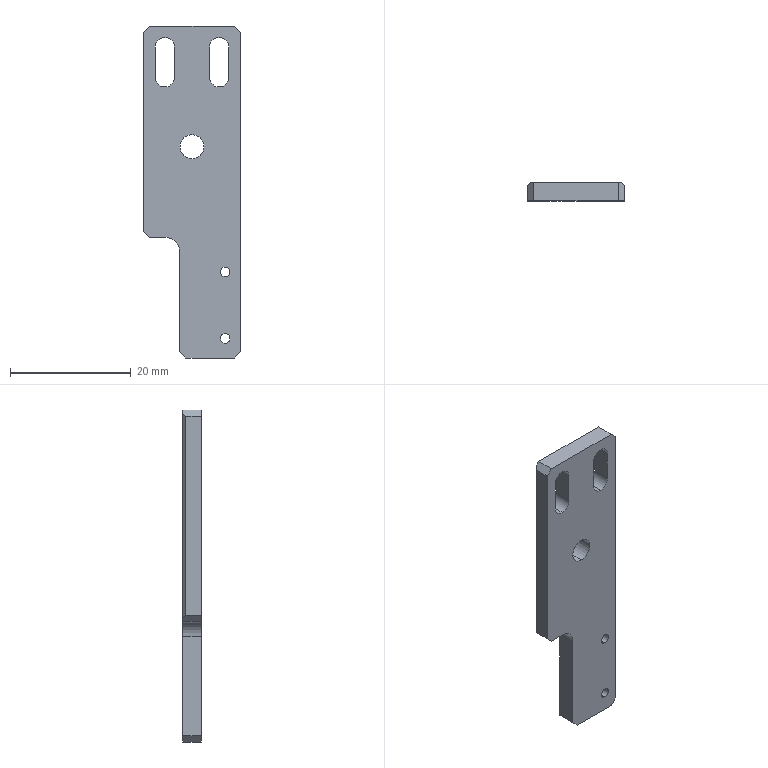Part | SolidWorks | features Chamfer 2, HoleWzd 2, Cut 1, Extrusion 1, Fillet 1, ICE 1 | 1 solid | 32 faces | box 16 x 3 x 55 mm | volume 2072 mm3 | plane 19 | cylinder 13 | commonest cylinder face diameters 3.2 x6 1.6 x4 4 x2 5 x1
STEP:
#1=CARTESIAN_POINT('',(8.,3.,33.));
#2=VERTEX_POINT('',#1);
#3=CARTESIAN_POINT('',(8.,3.,37.));
#4=VERTEX_POINT('',#3);
#5=CARTESIAN_POINT('',(8.,3.,35.));
#6=DIRECTION('',(0.,1.,0.));
#7=DIRECTION('',(0.,0.,1.));
#8=AXIS2_PLACEMENT_3D('',#5,#6,#7);
#9=CIRCLE('',#8,2.);
#10=EDGE_CURVE('',#2,#4,#9,.T.);
#11=ORIENTED_EDGE('',*,*,#10,.T.);
#12=CARTESIAN_POINT('',(8.,0.,37.));
#13=VERTEX_POINT('',#12);
#14=CARTESIAN_POINT('',(8.,0.,37.));
#15=DIRECTION('',(0.,-1.,0.));
#16=VECTOR('',#15,1000.);
#17=LINE('',#14,#16);
#18=EDGE_CURVE('',#4,#13,#17,.T.);
#19=ORIENTED_EDGE('',*,*,#18,.T.);
#20=CARTESIAN_POINT('',(8.,0.,33.));
#21=VERTEX_POINT('',#20);
#22=CARTESIAN_POINT('',(8.,0.,35.));
#23=DIRECTION('',(0.,-1.,0.));
#24=DIRECTION('',(0.,0.,-1.));
#25=AXIS2_PLACEMENT_3D('',#22,#23,#24);
#26=CIRCLE('',#25,2.);
#27=EDGE_CURVE('',#13,#21,#26,.T.);
#28=ORIENTED_EDGE('',*,*,#27,.T.);
#29=CARTESIAN_POINT('',(8.,0.,33.));
#30=DIRECTION('',(0.,-1.,0.));
#31=VECTOR('',#30,1000.);
#32=LINE('',#29,#31);
#33=EDGE_CURVE('',#2,#21,#32,.T.);
#34=ORIENTED_EDGE('',*,*,#33,.F.);
#35=EDGE_LOOP('',(#11,#19,#28,#34));
#36=FACE_OUTER_BOUND('',#35,.T.);
#37=CARTESIAN_POINT('',(8.,0.,35.));
#38=DIRECTION('',(0.,-1.,0.));
#39=DIRECTION('',(0.,0.,-1.));
#40=AXIS2_PLACEMENT_3D('',#37,#38,#39);
#41=CYLINDRICAL_SURFACE('',#40,2.);
#42=ADVANCED_FACE('',(#36),#41,.F.);
#43=CARTESIAN_POINT('',(13.5,0.,2.45));
#44=VERTEX_POINT('',#43);
#45=CARTESIAN_POINT('',(13.5,0.,4.05));
#46=VERTEX_POINT('',#45);
#47=CARTESIAN_POINT('',(13.5,0.,3.25));
#48=DIRECTION('',(0.,1.,0.));
#49=DIRECTION('',(0.,0.,1.));
#50=AXIS2_PLACEMENT_3D('',#47,#48,#49);
#51=CIRCLE('',#50,0.8);
#52=EDGE_CURVE('',#44,#46,#51,.T.);
#53=ORIENTED_EDGE('',*,*,#52,.F.);
#54=CARTESIAN_POINT('',(13.5,3.,2.45));
#55=VERTEX_POINT('',#54);
#56=CARTESIAN_POINT('',(13.5,3.,2.45));
#57=DIRECTION('',(0.,1.,0.));
#58=VECTOR('',#57,1000.);
#59=LINE('',#56,#58);
#60=EDGE_CURVE('',#44,#55,#59,.T.);
#61=ORIENTED_EDGE('',*,*,#60,.T.);
#62=CARTESIAN_POINT('',(13.5,3.,4.05));
#63=VERTEX_POINT('',#62);
#64=CARTESIAN_POINT('',(13.5,3.,3.25));
#65=DIRECTION('',(0.,1.,0.));
#66=DIRECTION('',(0.,0.,1.));
#67=AXIS2_PLACEMENT_3D('',#64,#65,#66);
#68=CIRCLE('',#67,0.8);
#69=EDGE_CURVE('',#55,#63,#68,.T.);
#70=ORIENTED_EDGE('',*,*,#69,.T.);
#71=CARTESIAN_POINT('',(13.5,3.,4.05));
#72=DIRECTION('',(0.,1.,0.));
#73=VECTOR('',#72,1000.);
#74=LINE('',#71,#73);
#75=EDGE_CURVE('',#46,#63,#74,.T.);
#76=ORIENTED_EDGE('',*,*,#75,.F.);
#77=EDGE_LOOP('',(#53,#61,#70,#76));
#78=FACE_OUTER_BOUND('',#77,.T.);
#79=CARTESIAN_POINT('',(13.5,3.,3.25));
#80=DIRECTION('',(0.,1.,0.));
#81=DIRECTION('',(0.,0.,1.));
#82=AXIS2_PLACEMENT_3D('',#79,#80,#81);
#83=CYLINDRICAL_SURFACE('',#82,0.8);
#84=ADVANCED_FACE('',(#78),#83,.F.);
#85=CARTESIAN_POINT('',(13.5,0.,13.45));
#86=VERTEX_POINT('',#85);
#87=CARTESIAN_POINT('',(13.5,0.,15.05));
#88=VERTEX_POINT('',#87);
#89=CARTESIAN_POINT('',(13.5,0.,14.25));
#90=DIRECTION('',(0.,1.,0.));
#91=DIRECTION('',(0.,0.,1.));
#92=AXIS2_PLACEMENT_3D('',#89,#90,#91);
#93=CIRCLE('',#92,0.8);
#94=EDGE_CURVE('',#86,#88,#93,.T.);
#95=ORIENTED_EDGE('',*,*,#94,.F.);
#96=CARTESIAN_POINT('',(13.5,3.,13.45));
#97=VERTEX_POINT('',#96);
#98=CARTESIAN_POINT('',(13.5,3.,13.45));
#99=DIRECTION('',(0.,1.,0.));
#100=VECTOR('',#99,1000.);
#101=LINE('',#98,#100);
#102=EDGE_CURVE('',#86,#97,#101,.T.);
#103=ORIENTED_EDGE('',*,*,#102,.T.);
#104=CARTESIAN_POINT('',(13.5,3.,15.05));
#105=VERTEX_POINT('',#104);
#106=CARTESIAN_POINT('',(13.5,3.,14.25));
#107=DIRECTION('',(0.,1.,0.));
#108=DIRECTION('',(0.,0.,1.));
#109=AXIS2_PLACEMENT_3D('',#106,#107,#108);
#110=CIRCLE('',#109,0.8);
#111=EDGE_CURVE('',#97,#105,#110,.T.);
#112=ORIENTED_EDGE('',*,*,#111,.T.);
#113=CARTESIAN_POINT('',(13.5,3.,15.05));
#114=DIRECTION('',(0.,1.,0.));
#115=VECTOR('',#114,1000.);
#116=LINE('',#113,#115);
#117=EDGE_CURVE('',#88,#105,#116,.T.);
#118=ORIENTED_EDGE('',*,*,#117,.F.);
#119=EDGE_LOOP('',(#95,#103,#112,#118));
#120=FACE_OUTER_BOUND('',#119,.T.);
#121=CARTESIAN_POINT('',(13.5,3.,14.25));
#122=DIRECTION('',(0.,1.,0.));
#123=DIRECTION('',(0.,0.,1.));
#124=AXIS2_PLACEMENT_3D('',#121,#122,#123);
#125=CYLINDRICAL_SURFACE('',#124,0.8);
#126=ADVANCED_FACE('',(#120),#125,.F.);
#127=CARTESIAN_POINT('',(14.1,3.,46.5));
#128=VERTEX_POINT('',#127);
#129=CARTESIAN_POINT('',(12.5,3.,44.9));
#130=VERTEX_POINT('',#129);
#131=CARTESIAN_POINT('',(12.5,3.,46.5));
#132=DIRECTION('',(0.,1.,0.));
#133=DIRECTION('',(0.,0.,1.));
#134=AXIS2_PLACEMENT_3D('',#131,#132,#133);
#135=CIRCLE('',#134,1.6);
#136=EDGE_CURVE('',#128,#130,#135,.T.);
#137=ORIENTED_EDGE('',*,*,#136,.T.);
#138=CARTESIAN_POINT('',(12.5,0.,44.9));
#139=VERTEX_POINT('',#138);
#140=CARTESIAN_POINT('',(12.5,10.,44.9));
#141=DIRECTION('',(0.,-1.,0.));
#142=VECTOR('',#141,1000.);
#143=LINE('',#140,#142);
#144=EDGE_CURVE('',#130,#139,#143,.T.);
#145=ORIENTED_EDGE('',*,*,#144,.T.);
#146=CARTESIAN_POINT('',(14.1,0.,46.5));
#147=VERTEX_POINT('',#146);
#148=CARTESIAN_POINT('',(12.5,0.,46.5));
#149=DIRECTION('',(0.,-1.,0.));
#150=DIRECTION('',(0.,0.,1.));
#151=AXIS2_PLACEMENT_3D('',#148,#149,#150);
#152=CIRCLE('',#151,1.6);
#153=EDGE_CURVE('',#139,#147,#152,.T.);
#154=ORIENTED_EDGE('',*,*,#153,.T.);
#155=CARTESIAN_POINT('',(14.1,10.,46.5));
#156=DIRECTION('',(0.,-1.,0.));
#157=VECTOR('',#156,1000.);
#158=LINE('',#155,#157);
#159=EDGE_CURVE('',#128,#147,#158,.T.);
#160=ORIENTED_EDGE('',*,*,#159,.F.);
#161=EDGE_LOOP('',(#137,#145,#154,#160));
#162=FACE_OUTER_BOUND('',#161,.T.);
#163=CARTESIAN_POINT('',(12.5,10.,46.5));
#164=DIRECTION('',(0.,-1.,0.));
#165=DIRECTION('',(0.,0.,-1.));
#166=AXIS2_PLACEMENT_3D('',#163,#164,#165);
#167=CYLINDRICAL_SURFACE('',#166,1.6);
#168=ADVANCED_FACE('',(#162),#167,.F.);
#169=CARTESIAN_POINT('',(5.1,3.,46.5));
#170=VERTEX_POINT('',#169);
#171=CARTESIAN_POINT('',(3.5,3.,44.9));
#172=VERTEX_POINT('',#171);
#173=CARTESIAN_POINT('',(3.5,3.,46.5));
#174=DIRECTION('',(0.,1.,0.));
#175=DIRECTION('',(0.,0.,1.));
#176=AXIS2_PLACEMENT_3D('',#173,#174,#175);
#177=CIRCLE('',#176,1.6);
#178=EDGE_CURVE('',#170,#172,#177,.T.);
#179=ORIENTED_EDGE('',*,*,#178,.T.);
#180=CARTESIAN_POINT('',(3.5,0.,44.9));
#181=VERTEX_POINT('',#180);
#182=CARTESIAN_POINT('',(3.5,10.,44.9));
#183=DIRECTION('',(0.,-1.,0.));
#184=VECTOR('',#183,1000.);
#185=LINE('',#182,#184);
#186=EDGE_CURVE('',#172,#181,#185,.T.);
#187=ORIENTED_EDGE('',*,*,#186,.T.);
#188=CARTESIAN_POINT('',(5.1,0.,46.5));
#189=VERTEX_POINT('',#188);
#190=CARTESIAN_POINT('',(3.5,0.,46.5));
#191=DIRECTION('',(0.,-1.,0.));
#192=DIRECTION('',(0.,0.,-1.));
#193=AXIS2_PLACEMENT_3D('',#190,#191,#192);
#194=CIRCLE('',#193,1.6);
#195=EDGE_CURVE('',#181,#189,#194,.T.);
#196=ORIENTED_EDGE('',*,*,#195,.T.);
#197=CARTESIAN_POINT('',(5.1,10.,46.5));
#198=DIRECTION('',(0.,-1.,0.));
#199=VECTOR('',#198,1000.);
#200=LINE('',#197,#199);
#201=EDGE_CURVE('',#170,#189,#200,.T.);
#202=ORIENTED_EDGE('',*,*,#201,.F.);
#203=EDGE_LOOP('',(#179,#187,#196,#202));
#204=FACE_OUTER_BOUND('',#203,.T.);
#205=CARTESIAN_POINT('',(3.5,10.,46.5));
#206=DIRECTION('',(0.,-1.,0.));
#207=DIRECTION('',(0.,0.,-1.));
#208=AXIS2_PLACEMENT_3D('',#205,#206,#207);
#209=CYLINDRICAL_SURFACE('',#208,1.6);
#210=ADVANCED_FACE('',(#204),#209,.F.);
#211=CARTESIAN_POINT('',(0.,0.,54.));
#212=VERTEX_POINT('',#211);
#213=CARTESIAN_POINT('',(0.,2.5,54.));
#214=VERTEX_POINT('',#213);
#215=CARTESIAN_POINT('',(0.,3.,54.));
#216=DIRECTION('',(0.,1.,0.));
#217=VECTOR('',#216,1000.);
#218=LINE('',#215,#217);
#219=EDGE_CURVE('',#212,#214,#218,.T.);
#220=ORIENTED_EDGE('',*,*,#219,.T.);
#221=CARTESIAN_POINT('',(0.,2.5,21.));
#222=VERTEX_POINT('',#221);
#223=CARTESIAN_POINT('',(0.,2.5,21.));
#224=DIRECTION('',(0.,0.,-1.));
#225=VECTOR('',#224,1000.);
#226=LINE('',#223,#225);
#227=EDGE_CURVE('',#214,#222,#226,.T.);
#228=ORIENTED_EDGE('',*,*,#227,.T.);
#229=CARTESIAN_POINT('',(0.,0.,21.));
#230=VERTEX_POINT('',#229);
#231=CARTESIAN_POINT('',(0.,3.,21.));
#232=DIRECTION('',(0.,-1.,0.));
#233=VECTOR('',#232,1000.);
#234=LINE('',#231,#233);
#235=EDGE_CURVE('',#222,#230,#234,.T.);
#236=ORIENTED_EDGE('',*,*,#235,.T.);
#237=CARTESIAN_POINT('',(0.,0.,0.));
#238=DIRECTION('',(0.,0.,1.));
#239=VECTOR('',#238,1000.);
#240=LINE('',#237,#239);
#241=EDGE_CURVE('',#230,#212,#240,.T.);
#242=ORIENTED_EDGE('',*,*,#241,.T.);
#243=EDGE_LOOP('',(#220,#228,#236,#242));
#244=FACE_OUTER_BOUND('',#243,.T.);
#245=CARTESIAN_POINT('',(0.,3.,0.));
#246=DIRECTION('',(1.,0.,0.));
#247=DIRECTION('',(0.,0.,-1.));
#248=AXIS2_PLACEMENT_3D('',#245,#246,#247);
#249=PLANE('',#248);
#250=ADVANCED_FACE('',(#244),#249,.F.);
#251=CARTESIAN_POINT('',(1.,0.,55.));
#252=VERTEX_POINT('',#251);
#253=CARTESIAN_POINT('',(15.,0.,55.));
#254=VERTEX_POINT('',#253);
#255=CARTESIAN_POINT('',(0.,0.,55.));
#256=DIRECTION('',(1.,0.,0.));
#257=VECTOR('',#256,1000.);
#258=LINE('',#255,#257);
#259=EDGE_CURVE('',#252,#254,#258,.T.);
#260=ORIENTED_EDGE('',*,*,#259,.T.);
#261=CARTESIAN_POINT('',(15.,3.,55.));
#262=VERTEX_POINT('',#261);
#263=CARTESIAN_POINT('',(15.,3.,55.));
#264=DIRECTION('',(0.,1.,0.));
#265=VECTOR('',#264,1000.);
#266=LINE('',#263,#265);
#267=EDGE_CURVE('',#254,#262,#266,.T.);
#268=ORIENTED_EDGE('',*,*,#267,.T.);
#269=CARTESIAN_POINT('',(1.,3.,55.));
#270=VERTEX_POINT('',#269);
#271=CARTESIAN_POINT('',(0.,3.,55.));
#272=DIRECTION('',(1.,0.,0.));
#273=VECTOR('',#272,1000.);
#274=LINE('',#271,#273);
#275=EDGE_CURVE('',#270,#262,#274,.T.);
#276=ORIENTED_EDGE('',*,*,#275,.F.);
#277=CARTESIAN_POINT('',(1.,3.,55.));
#278=DIRECTION('',(0.,-1.,0.));
#279=VECTOR('',#278,1000.);
#280=LINE('',#277,#279);
#281=EDGE_CURVE('',#270,#252,#280,.T.);
#282=ORIENTED_EDGE('',*,*,#281,.T.);
#283=EDGE_LOOP('',(#260,#268,#276,#282));
#284=FACE_OUTER_BOUND('',#283,.T.);
#285=CARTESIAN_POINT('',(0.,3.,55.));
#286=DIRECTION('',(0.,0.,-1.));
#287=DIRECTION('',(-1.,0.,0.));
#288=AXIS2_PLACEMENT_3D('',#285,#286,#287);
#289=PLANE('',#288);
#290=ADVANCED_FACE('',(#284),#289,.F.);
#291=CARTESIAN_POINT('',(16.,0.,1.));
#292=VERTEX_POINT('',#291);
#293=CARTESIAN_POINT('',(16.,2.5,1.));
#294=VERTEX_POINT('',#293);
#295=CARTESIAN_POINT('',(16.,3.,1.));
#296=DIRECTION('',(0.,1.,0.));
#297=VECTOR('',#296,1000.);
#298=LINE('',#295,#297);
#299=EDGE_CURVE('',#292,#294,#298,.T.);
#300=ORIENTED_EDGE('',*,*,#299,.T.);
#301=CARTESIAN_POINT('',(16.,2.5,54.));
#302=VERTEX_POINT('',#301);
#303=CARTESIAN_POINT('',(16.,2.5,54.));
#304=DIRECTION('',(0.,0.,1.));
#305=VECTOR('',#304,1000.);
#306=LINE('',#303,#305);
#307=EDGE_CURVE('',#294,#302,#306,.T.);
#308=ORIENTED_EDGE('',*,*,#307,.T.);
#309=CARTESIAN_POINT('',(16.,0.,54.));
#310=VERTEX_POINT('',#309);
#311=CARTESIAN_POINT('',(16.,3.,54.));
#312=DIRECTION('',(0.,-1.,0.));
#313=VECTOR('',#312,1000.);
#314=LINE('',#311,#313);
#315=EDGE_CURVE('',#302,#310,#314,.T.);
#316=ORIENTED_EDGE('',*,*,#315,.T.);
#317=CARTESIAN_POINT('',(16.,0.,0.));
#318=DIRECTION('',(0.,0.,-1.));
#319=VECTOR('',#318,1000.);
#320=LINE('',#317,#319);
#321=EDGE_CURVE('',#310,#292,#320,.T.);
#322=ORIENTED_EDGE('',*,*,#321,.T.);
#323=EDGE_LOOP('',(#300,#308,#316,#322));
#324=FACE_OUTER_BOUND('',#323,.T.);
#325=CARTESIAN_POINT('',(16.,3.,0.));
#326=DIRECTION('',(-1.,0.,0.));
#327=DIRECTION('',(0.,0.,1.));
#328=AXIS2_PLACEMENT_3D('',#325,#326,#327);
#329=PLANE('',#328);
#330=ADVANCED_FACE('',(#324),#329,.F.);
#331=CARTESIAN_POINT('',(15.,0.,0.));
#332=VERTEX_POINT('',#331);
#333=CARTESIAN_POINT('',(7.,0.,0.));
#334=VERTEX_POINT('',#333);
#335=CARTESIAN_POINT('',(0.,0.,0.));
#336=DIRECTION('',(-1.,0.,0.));
#337=VECTOR('',#336,1000.);
#338=LINE('',#335,#337);
#339=EDGE_CURVE('',#332,#334,#338,.T.);
#340=ORIENTED_EDGE('',*,*,#339,.T.);
#341=CARTESIAN_POINT('',(7.,3.,0.));
#342=VERTEX_POINT('',#341);
#343=CARTESIAN_POINT('',(7.,3.,0.));
#344=DIRECTION('',(0.,1.,0.));
#345=VECTOR('',#344,1000.);
#346=LINE('',#343,#345);
#347=EDGE_CURVE('',#334,#342,#346,.T.);
#348=ORIENTED_EDGE('',*,*,#347,.T.);
#349=CARTESIAN_POINT('',(15.,3.,0.));
#350=VERTEX_POINT('',#349);
#351=CARTESIAN_POINT('',(0.,3.,0.));
#352=DIRECTION('',(-1.,0.,0.));
#353=VECTOR('',#352,1000.);
#354=LINE('',#351,#353);
#355=EDGE_CURVE('',#350,#342,#354,.T.);
#356=ORIENTED_EDGE('',*,*,#355,.F.);
#357=CARTESIAN_POINT('',(15.,3.,0.));
#358=DIRECTION('',(0.,-1.,0.));
#359=VECTOR('',#358,1000.);
#360=LINE('',#357,#359);
#361=EDGE_CURVE('',#350,#332,#360,.T.);
#362=ORIENTED_EDGE('',*,*,#361,.T.);
#363=EDGE_LOOP('',(#340,#348,#356,#362));
#364=FACE_OUTER_BOUND('',#363,.T.);
#365=CARTESIAN_POINT('',(0.,3.,0.));
#366=DIRECTION('',(0.,0.,1.));
#367=DIRECTION('',(1.,0.,0.));
#368=AXIS2_PLACEMENT_3D('',#365,#366,#367);
#369=PLANE('',#368);
#370=ADVANCED_FACE('',(#364),#369,.F.);
#371=ORIENTED_EDGE('',*,*,#10,.F.);
#372=CARTESIAN_POINT('',(8.,3.,35.));
#373=DIRECTION('',(0.,1.,0.));
#374=DIRECTION('',(0.,0.,1.));
#375=AXIS2_PLACEMENT_3D('',#372,#373,#374);
#376=CIRCLE('',#375,2.);
#377=EDGE_CURVE('',#4,#2,#376,.T.);
#378=ORIENTED_EDGE('',*,*,#377,.F.);
#379=EDGE_LOOP('',(#371,#378));
#380=FACE_BOUND('',#379,.T.);
#381=CARTESIAN_POINT('',(13.5,3.,3.25));
#382=DIRECTION('',(0.,1.,0.));
#383=DIRECTION('',(0.,0.,1.));
#384=AXIS2_PLACEMENT_3D('',#381,#382,#383);
#385=CIRCLE('',#384,0.8);
#386=EDGE_CURVE('',#63,#55,#385,.T.);
#387=ORIENTED_EDGE('',*,*,#386,.F.);
#388=ORIENTED_EDGE('',*,*,#69,.F.);
#389=EDGE_LOOP('',(#387,#388));
#390=FACE_BOUND('',#389,.T.);
#391=CARTESIAN_POINT('',(13.5,3.,14.25));
#392=DIRECTION('',(0.,1.,0.));
#393=DIRECTION('',(0.,0.,1.));
#394=AXIS2_PLACEMENT_3D('',#391,#392,#393);
#395=CIRCLE('',#394,0.8);
#396=EDGE_CURVE('',#105,#97,#395,.T.);
#397=ORIENTED_EDGE('',*,*,#396,.F.);
#398=ORIENTED_EDGE('',*,*,#111,.F.);
#399=EDGE_LOOP('',(#397,#398));
#400=FACE_BOUND('',#399,.T.);
#401=CARTESIAN_POINT('',(15.5,3.,54.5));
#402=VERTEX_POINT('',#401);
#403=CARTESIAN_POINT('',(35.,3.,35.));
#404=DIRECTION('',(0.7071,0.,-0.7071));
#405=VECTOR('',#404,1000.);
#406=LINE('',#403,#405);
#407=EDGE_CURVE('',#262,#402,#406,.T.);
#408=ORIENTED_EDGE('',*,*,#407,.T.);
#409=CARTESIAN_POINT('',(15.5,3.,0.5));
#410=VERTEX_POINT('',#409);
#411=CARTESIAN_POINT('',(15.5,3.,1.));
#412=DIRECTION('',(0.,0.,-1.));
#413=VECTOR('',#412,1000.);
#414=LINE('',#411,#413);
#415=EDGE_CURVE('',#402,#410,#414,.T.);
#416=ORIENTED_EDGE('',*,*,#415,.T.);
#417=CARTESIAN_POINT('',(7.5,3.,-7.5));
#418=DIRECTION('',(-0.7071,0.,-0.7071));
#419=VECTOR('',#418,1000.);
#420=LINE('',#417,#419);
#421=EDGE_CURVE('',#410,#350,#420,.T.);
#422=ORIENTED_EDGE('',*,*,#421,.T.);
#423=ORIENTED_EDGE('',*,*,#355,.T.);
#424=CARTESIAN_POINT('',(6.,3.,1.));
#425=VERTEX_POINT('',#424);
#426=CARTESIAN_POINT('',(3.5,3.,3.5));
#427=DIRECTION('',(-0.7071,0.,0.7071));
#428=VECTOR('',#427,1000.);
#429=LINE('',#426,#428);
#430=EDGE_CURVE('',#342,#425,#429,.T.);
#431=ORIENTED_EDGE('',*,*,#430,.T.);
#432=CARTESIAN_POINT('',(6.,3.,17.5));
#433=VERTEX_POINT('',#432);
#434=CARTESIAN_POINT('',(6.,3.,0.));
#435=DIRECTION('',(0.,0.,-1.));
#436=VECTOR('',#435,1000.);
#437=LINE('',#434,#436);
#438=EDGE_CURVE('',#433,#425,#437,.T.);
#439=ORIENTED_EDGE('',*,*,#438,.F.);
#440=CARTESIAN_POINT('',(3.5,3.,20.));
#441=VERTEX_POINT('',#440);
#442=CARTESIAN_POINT('',(3.5,3.,17.5));
#443=DIRECTION('',(0.,-1.,0.));
#444=DIRECTION('',(0.,0.,1.));
#445=AXIS2_PLACEMENT_3D('',#442,#443,#444);
#446=CIRCLE('',#445,2.5);
#447=EDGE_CURVE('',#433,#441,#446,.T.);
#448=ORIENTED_EDGE('',*,*,#447,.T.);
#449=CARTESIAN_POINT('',(1.,3.,20.));
#450=VERTEX_POINT('',#449);
#451=CARTESIAN_POINT('',(0.,3.,20.));
#452=DIRECTION('',(1.,0.,0.));
#453=VECTOR('',#452,1000.);
#454=LINE('',#451,#453);
#455=EDGE_CURVE('',#450,#441,#454,.T.);
#456=ORIENTED_EDGE('',*,*,#455,.F.);
#457=CARTESIAN_POINT('',(0.5,3.,20.5));
#458=VERTEX_POINT('',#457);
#459=CARTESIAN_POINT('',(10.5,3.,10.5));
#460=DIRECTION('',(-0.7071,0.,0.7071));
#461=VECTOR('',#460,1000.);
#462=LINE('',#459,#461);
#463=EDGE_CURVE('',#450,#458,#462,.T.);
#464=ORIENTED_EDGE('',*,*,#463,.T.);
#465=CARTESIAN_POINT('',(0.5,3.,54.5));
#466=VERTEX_POINT('',#465);
#467=CARTESIAN_POINT('',(0.5,3.,54.));
#468=DIRECTION('',(0.,0.,1.));
#469=VECTOR('',#468,1000.);
#470=LINE('',#467,#469);
#471=EDGE_CURVE('',#458,#466,#470,.T.);
#472=ORIENTED_EDGE('',*,*,#471,.T.);
#473=CARTESIAN_POINT('',(-27.,3.,27.));
#474=DIRECTION('',(0.7071,0.,0.7071));
#475=VECTOR('',#474,1000.);
#476=LINE('',#473,#475);
#477=EDGE_CURVE('',#466,#270,#476,.T.);
#478=ORIENTED_EDGE('',*,*,#477,.T.);
#479=ORIENTED_EDGE('',*,*,#275,.T.);
#480=EDGE_LOOP('',(#408,#416,#422,#423,#431,#439,#448,#456,#464,#472,#478,#479));
#481=FACE_OUTER_BOUND('',#480,.T.);
#482=CARTESIAN_POINT('',(10.9,3.,51.5));
#483=VERTEX_POINT('',#482);
#484=CARTESIAN_POINT('',(14.1,3.,51.5));
#485=VERTEX_POINT('',#484);
#486=CARTESIAN_POINT('',(12.5,3.,51.5));
#487=DIRECTION('',(0.,1.,0.));
#488=DIRECTION('',(0.,0.,1.));
#489=AXIS2_PLACEMENT_3D('',#486,#487,#488);
#490=CIRCLE('',#489,1.6);
#491=EDGE_CURVE('',#483,#485,#490,.T.);
#492=ORIENTED_EDGE('',*,*,#491,.F.);
#493=CARTESIAN_POINT('',(10.9,3.,46.5));
#494=VERTEX_POINT('',#493);
#495=CARTESIAN_POINT('',(10.9,3.,0.));
#496=DIRECTION('',(0.,0.,1.));
#497=VECTOR('',#496,1000.);
#498=LINE('',#495,#497);
#499=EDGE_CURVE('',#494,#483,#498,.T.);
#500=ORIENTED_EDGE('',*,*,#499,.F.);
#501=CARTESIAN_POINT('',(12.5,3.,46.5));
#502=DIRECTION('',(0.,1.,0.));
#503=DIRECTION('',(0.,0.,1.));
#504=AXIS2_PLACEMENT_3D('',#501,#502,#503);
#505=CIRCLE('',#504,1.6);
#506=EDGE_CURVE('',#130,#494,#505,.T.);
#507=ORIENTED_EDGE('',*,*,#506,.F.);
#508=ORIENTED_EDGE('',*,*,#136,.F.);
#509=CARTESIAN_POINT('',(14.1,3.,0.));
#510=DIRECTION('',(0.,0.,-1.));
#511=VECTOR('',#510,1000.);
#512=LINE('',#509,#511);
#513=EDGE_CURVE('',#485,#128,#512,.T.);
#514=ORIENTED_EDGE('',*,*,#513,.F.);
#515=EDGE_LOOP('',(#492,#500,#507,#508,#514));
#516=FACE_BOUND('',#515,.T.);
#517=CARTESIAN_POINT('',(1.9,3.,51.5));
#518=VERTEX_POINT('',#517);
#519=CARTESIAN_POINT('',(5.1,3.,51.5));
#520=VERTEX_POINT('',#519);
#521=CARTESIAN_POINT('',(3.5,3.,51.5));
#522=DIRECTION('',(0.,1.,0.));
#523=DIRECTION('',(0.,0.,1.));
#524=AXIS2_PLACEMENT_3D('',#521,#522,#523);
#525=CIRCLE('',#524,1.6);
#526=EDGE_CURVE('',#518,#520,#525,.T.);
#527=ORIENTED_EDGE('',*,*,#526,.F.);
#528=CARTESIAN_POINT('',(1.9,3.,46.5));
#529=VERTEX_POINT('',#528);
#530=CARTESIAN_POINT('',(1.9,3.,0.));
#531=DIRECTION('',(0.,0.,1.));
#532=VECTOR('',#531,1000.);
#533=LINE('',#530,#532);
#534=EDGE_CURVE('',#529,#518,#533,.T.);
#535=ORIENTED_EDGE('',*,*,#534,.F.);
#536=CARTESIAN_POINT('',(3.5,3.,46.5));
#537=DIRECTION('',(0.,1.,0.));
#538=DIRECTION('',(0.,0.,1.));
#539=AXIS2_PLACEMENT_3D('',#536,#537,#538);
#540=CIRCLE('',#539,1.6);
#541=EDGE_CURVE('',#172,#529,#540,.T.);
#542=ORIENTED_EDGE('',*,*,#541,.F.);
#543=ORIENTED_EDGE('',*,*,#178,.F.);
#544=CARTESIAN_POINT('',(5.1,3.,0.));
#545=DIRECTION('',(0.,0.,-1.));
#546=VECTOR('',#545,1000.);
#547=LINE('',#544,#546);
#548=EDGE_CURVE('',#520,#170,#547,.T.);
#549=ORIENTED_EDGE('',*,*,#548,.F.);
#550=EDGE_LOOP('',(#527,#535,#542,#543,#549));
#551=FACE_BOUND('',#550,.T.);
#552=CARTESIAN_POINT('',(0.,3.,0.));
#553=DIRECTION('',(0.,1.,0.));
#554=DIRECTION('',(0.,0.,1.));
#555=AXIS2_PLACEMENT_3D('',#552,#553,#554);
#556=PLANE('',#555);
#557=ADVANCED_FACE('',(#380,#390,#400,#481,#516,#551),#556,.T.);
#558=CARTESIAN_POINT('',(8.,0.,35.));
#559=DIRECTION('',(0.,-1.,0.));
#560=DIRECTION('',(0.,0.,-1.));
#561=AXIS2_PLACEMENT_3D('',#558,#559,#560);
#562=CIRCLE('',#561,2.);
#563=EDGE_CURVE('',#21,#13,#562,.T.);
#564=ORIENTED_EDGE('',*,*,#563,.F.);
#565=ORIENTED_EDGE('',*,*,#27,.F.);
#566=EDGE_LOOP('',(#564,#565));
#567=FACE_BOUND('',#566,.T.);
#568=CARTESIAN_POINT('',(13.5,0.,3.25));
#569=DIRECTION('',(0.,1.,0.));
#570=DIRECTION('',(0.,0.,1.));
#571=AXIS2_PLACEMENT_3D('',#568,#569,#570);
#572=CIRCLE('',#571,0.8);
#573=EDGE_CURVE('',#46,#44,#572,.T.);
#574=ORIENTED_EDGE('',*,*,#573,.T.);
#575=ORIENTED_EDGE('',*,*,#52,.T.);
#576=EDGE_LOOP('',(#574,#575));
#577=FACE_BOUND('',#576,.T.);
#578=CARTESIAN_POINT('',(13.5,0.,14.25));
#579=DIRECTION('',(0.,1.,0.));
#580=DIRECTION('',(0.,0.,1.));
#581=AXIS2_PLACEMENT_3D('',#578,#579,#580);
#582=CIRCLE('',#581,0.8);
#583=EDGE_CURVE('',#88,#86,#582,.T.);
#584=ORIENTED_EDGE('',*,*,#583,.T.);
#585=ORIENTED_EDGE('',*,*,#94,.T.);
#586=EDGE_LOOP('',(#584,#585));
#587=FACE_BOUND('',#586,.T.);
#588=CARTESIAN_POINT('',(10.9,0.,51.5));
#589=VERTEX_POINT('',#588);
#590=CARTESIAN_POINT('',(10.9,0.,46.5));
#591=VERTEX_POINT('',#590);
#592=CARTESIAN_POINT('',(10.9,0.,51.5));
#593=DIRECTION('',(0.,0.,-1.));
#594=VECTOR('',#593,1000.);
#595=LINE('',#592,#594);
#596=EDGE_CURVE('',#589,#591,#595,.T.);
#597=ORIENTED_EDGE('',*,*,#596,.F.);
#598=CARTESIAN_POINT('',(14.1,0.,51.5));
#599=VERTEX_POINT('',#598);
#600=CARTESIAN_POINT('',(12.5,0.,51.5));
#601=DIRECTION('',(0.,-1.,0.));
#602=DIRECTION('',(0.,0.,1.));
#603=AXIS2_PLACEMENT_3D('',#600,#601,#602);
#604=CIRCLE('',#603,1.6);
#605=EDGE_CURVE('',#599,#589,#604,.T.);
#606=ORIENTED_EDGE('',*,*,#605,.F.);
#607=CARTESIAN_POINT('',(14.1,0.,51.5));
#608=DIRECTION('',(0.,0.,1.));
#609=VECTOR('',#608,1000.);
#610=LINE('',#607,#609);
#611=EDGE_CURVE('',#147,#599,#610,.T.);
#612=ORIENTED_EDGE('',*,*,#611,.F.);
#613=ORIENTED_EDGE('',*,*,#153,.F.);
#614=CARTESIAN_POINT('',(12.5,0.,46.5));
#615=DIRECTION('',(0.,-1.,0.));
#616=DIRECTION('',(0.,0.,1.));
#617=AXIS2_PLACEMENT_3D('',#614,#615,#616);
#618=CIRCLE('',#617,1.6);
#619=EDGE_CURVE('',#591,#139,#618,.T.);
#620=ORIENTED_EDGE('',*,*,#619,.F.);
#621=EDGE_LOOP('',(#597,#606,#612,#613,#620));
#622=FACE_BOUND('',#621,.T.);
#623=CARTESIAN_POINT('',(1.9,0.,51.5));
#624=VERTEX_POINT('',#623);
#625=CARTESIAN_POINT('',(1.9,0.,46.5));
#626=VERTEX_POINT('',#625);
#627=CARTESIAN_POINT('',(1.9,0.,51.5));
#628=DIRECTION('',(0.,0.,-1.));
#629=VECTOR('',#628,1000.);
#630=LINE('',#627,#629);
#631=EDGE_CURVE('',#624,#626,#630,.T.);
#632=ORIENTED_EDGE('',*,*,#631,.F.);
#633=CARTESIAN_POINT('',(5.1,0.,51.5));
#634=VERTEX_POINT('',#633);
#635=CARTESIAN_POINT('',(3.5,0.,51.5));
#636=DIRECTION('',(0.,-1.,0.));
#637=DIRECTION('',(0.,0.,-1.));
#638=AXIS2_PLACEMENT_3D('',#635,#636,#637);
#639=CIRCLE('',#638,1.6);
#640=EDGE_CURVE('',#634,#624,#639,.T.);
#641=ORIENTED_EDGE('',*,*,#640,.F.);
#642=CARTESIAN_POINT('',(5.1,0.,51.5));
#643=DIRECTION('',(0.,0.,1.));
#644=VECTOR('',#643,1000.);
#645=LINE('',#642,#644);
#646=EDGE_CURVE('',#189,#634,#645,.T.);
#647=ORIENTED_EDGE('',*,*,#646,.F.);
#648=ORIENTED_EDGE('',*,*,#195,.F.);
#649=CARTESIAN_POINT('',(3.5,0.,46.5));
#650=DIRECTION('',(0.,-1.,0.));
#651=DIRECTION('',(0.,0.,-1.));
#652=AXIS2_PLACEMENT_3D('',#649,#650,#651);
#653=CIRCLE('',#652,1.6);
#654=EDGE_CURVE('',#626,#181,#653,.T.);
#655=ORIENTED_EDGE('',*,*,#654,.F.);
#656=EDGE_LOOP('',(#632,#641,#647,#648,#655));
#657=FACE_BOUND('',#656,.T.);
#658=ORIENTED_EDGE('',*,*,#241,.F.);
#659=CARTESIAN_POINT('',(1.,0.,20.));
#660=VERTEX_POINT('',#659);
#661=CARTESIAN_POINT('',(1.,0.,20.));
#662=DIRECTION('',(0.7071,0.,-0.7071));
#663=VECTOR('',#662,1000.);
#664=LINE('',#661,#663);
#665=EDGE_CURVE('',#230,#660,#664,.T.);
#666=ORIENTED_EDGE('',*,*,#665,.T.);
#667=CARTESIAN_POINT('',(3.5,0.,20.));
#668=VERTEX_POINT('',#667);
#669=CARTESIAN_POINT('',(0.,0.,20.));
#670=DIRECTION('',(1.,0.,0.));
#671=VECTOR('',#670,1000.);
#672=LINE('',#669,#671);
#673=EDGE_CURVE('',#660,#668,#672,.T.);
#674=ORIENTED_EDGE('',*,*,#673,.T.);
#675=CARTESIAN_POINT('',(6.,0.,17.5));
#676=VERTEX_POINT('',#675);
#677=CARTESIAN_POINT('',(3.5,0.,17.5));
#678=DIRECTION('',(0.,1.,0.));
#679=DIRECTION('',(0.,0.,1.));
#680=AXIS2_PLACEMENT_3D('',#677,#678,#679);
#681=CIRCLE('',#680,2.5);
#682=EDGE_CURVE('',#668,#676,#681,.T.);
#683=ORIENTED_EDGE('',*,*,#682,.T.);
#684=CARTESIAN_POINT('',(6.,0.,1.));
#685=VERTEX_POINT('',#684);
#686=CARTESIAN_POINT('',(6.,0.,0.));
#687=DIRECTION('',(0.,0.,-1.));
#688=VECTOR('',#687,1000.);
#689=LINE('',#686,#688);
#690=EDGE_CURVE('',#676,#685,#689,.T.);
#691=ORIENTED_EDGE('',*,*,#690,.T.);
#692=CARTESIAN_POINT('',(7.,0.,0.));
#693=DIRECTION('',(0.7071,0.,-0.7071));
#694=VECTOR('',#693,1000.);
#695=LINE('',#692,#694);
#696=EDGE_CURVE('',#685,#334,#695,.T.);
#697=ORIENTED_EDGE('',*,*,#696,.T.);
#698=ORIENTED_EDGE('',*,*,#339,.F.);
#699=CARTESIAN_POINT('',(15.,0.,0.));
#700=DIRECTION('',(0.7071,0.,0.7071));
#701=VECTOR('',#700,1000.);
#702=LINE('',#699,#701);
#703=EDGE_CURVE('',#332,#292,#702,.T.);
#704=ORIENTED_EDGE('',*,*,#703,.T.);
#705=ORIENTED_EDGE('',*,*,#321,.F.);
#706=CARTESIAN_POINT('',(16.,0.,54.));
#707=DIRECTION('',(-0.7071,0.,0.7071));
#708=VECTOR('',#707,1000.);
#709=LINE('',#706,#708);
#710=EDGE_CURVE('',#310,#254,#709,.T.);
#711=ORIENTED_EDGE('',*,*,#710,.T.);
#712=ORIENTED_EDGE('',*,*,#259,.F.);
#713=CARTESIAN_POINT('',(1.,0.,55.));
#714=DIRECTION('',(-0.7071,0.,-0.7071));
#715=VECTOR('',#714,1000.);
#716=LINE('',#713,#715);
#717=EDGE_CURVE('',#252,#212,#716,.T.);
#718=ORIENTED_EDGE('',*,*,#717,.T.);
#719=EDGE_LOOP('',(#658,#666,#674,#683,#691,#697,#698,#704,#705,#711,#712,#718));
#720=FACE_OUTER_BOUND('',#719,.T.);
#721=CARTESIAN_POINT('',(0.,0.,0.));
#722=DIRECTION('',(0.,1.,0.));
#723=DIRECTION('',(0.,0.,1.));
#724=AXIS2_PLACEMENT_3D('',#721,#722,#723);
#725=PLANE('',#724);
#726=ADVANCED_FACE('',(#567,#577,#587,#622,#657,#720),#725,.F.);
#727=ORIENTED_EDGE('',*,*,#526,.T.);
#728=CARTESIAN_POINT('',(5.1,10.,51.5));
#729=DIRECTION('',(0.,-1.,0.));
#730=VECTOR('',#729,1000.);
#731=LINE('',#728,#730);
#732=EDGE_CURVE('',#520,#634,#731,.T.);
#733=ORIENTED_EDGE('',*,*,#732,.T.);
#734=ORIENTED_EDGE('',*,*,#640,.T.);
#735=CARTESIAN_POINT('',(1.9,10.,51.5));
#736=DIRECTION('',(0.,-1.,0.));
#737=VECTOR('',#736,1000.);
#738=LINE('',#735,#737);
#739=EDGE_CURVE('',#518,#624,#738,.T.);
#740=ORIENTED_EDGE('',*,*,#739,.F.);
#741=EDGE_LOOP('',(#727,#733,#734,#740));
#742=FACE_OUTER_BOUND('',#741,.T.);
#743=CARTESIAN_POINT('',(3.5,10.,51.5));
#744=DIRECTION('',(0.,-1.,0.));
#745=DIRECTION('',(0.,0.,-1.));
#746=AXIS2_PLACEMENT_3D('',#743,#744,#745);
#747=CYLINDRICAL_SURFACE('',#746,1.6);
#748=ADVANCED_FACE('',(#742),#747,.F.);
#749=ORIENTED_EDGE('',*,*,#548,.T.);
#750=ORIENTED_EDGE('',*,*,#201,.T.);
#751=ORIENTED_EDGE('',*,*,#646,.T.);
#752=ORIENTED_EDGE('',*,*,#732,.F.);
#753=EDGE_LOOP('',(#749,#750,#751,#752));
#754=FACE_OUTER_BOUND('',#753,.T.);
#755=CARTESIAN_POINT('',(5.1,10.,51.5));
#756=DIRECTION('',(1.,0.,0.));
#757=DIRECTION('',(0.,0.,-1.));
#758=AXIS2_PLACEMENT_3D('',#755,#756,#757);
#759=PLANE('',#758);
#760=ADVANCED_FACE('',(#754),#759,.F.);
#761=ORIENTED_EDGE('',*,*,#186,.F.);
#762=ORIENTED_EDGE('',*,*,#541,.T.);
#763=CARTESIAN_POINT('',(1.9,10.,46.5));
#764=DIRECTION('',(0.,-1.,0.));
#765=VECTOR('',#764,1000.);
#766=LINE('',#763,#765);
#767=EDGE_CURVE('',#529,#626,#766,.T.);
#768=ORIENTED_EDGE('',*,*,#767,.T.);
#769=ORIENTED_EDGE('',*,*,#654,.T.);
#770=EDGE_LOOP('',(#761,#762,#768,#769));
#771=FACE_OUTER_BOUND('',#770,.T.);
#772=CARTESIAN_POINT('',(3.5,10.,46.5));
#773=DIRECTION('',(0.,-1.,0.));
#774=DIRECTION('',(0.,0.,-1.));
#775=AXIS2_PLACEMENT_3D('',#772,#773,#774);
#776=CYLINDRICAL_SURFACE('',#775,1.6);
#777=ADVANCED_FACE('',(#771),#776,.F.);
#778=ORIENTED_EDGE('',*,*,#534,.T.);
#779=ORIENTED_EDGE('',*,*,#739,.T.);
#780=ORIENTED_EDGE('',*,*,#631,.T.);
#781=ORIENTED_EDGE('',*,*,#767,.F.);
#782=EDGE_LOOP('',(#778,#779,#780,#781));
#783=FACE_OUTER_BOUND('',#782,.T.);
#784=CARTESIAN_POINT('',(1.9,10.,51.5));
#785=DIRECTION('',(-1.,0.,0.));
#786=DIRECTION('',(0.,0.,1.));
#787=AXIS2_PLACEMENT_3D('',#784,#785,#786);
#788=PLANE('',#787);
#789=ADVANCED_FACE('',(#783),#788,.F.);
#790=ORIENTED_EDGE('',*,*,#491,.T.);
#791=CARTESIAN_POINT('',(14.1,10.,51.5));
#792=DIRECTION('',(0.,-1.,0.));
#793=VECTOR('',#792,1000.);
#794=LINE('',#791,#793);
#795=EDGE_CURVE('',#485,#599,#794,.T.);
#796=ORIENTED_EDGE('',*,*,#795,.T.);
#797=ORIENTED_EDGE('',*,*,#605,.T.);
#798=CARTESIAN_POINT('',(10.9,10.,51.5));
#799=DIRECTION('',(0.,-1.,0.));
#800=VECTOR('',#799,1000.);
#801=LINE('',#798,#800);
#802=EDGE_CURVE('',#483,#589,#801,.T.);
#803=ORIENTED_EDGE('',*,*,#802,.F.);
#804=EDGE_LOOP('',(#790,#796,#797,#803));
#805=FACE_OUTER_BOUND('',#804,.T.);
#806=CARTESIAN_POINT('',(12.5,10.,51.5));
#807=DIRECTION('',(0.,-1.,0.));
#808=DIRECTION('',(0.,0.,-1.));
#809=AXIS2_PLACEMENT_3D('',#806,#807,#808);
#810=CYLINDRICAL_SURFACE('',#809,1.6);
#811=ADVANCED_FACE('',(#805),#810,.F.);
#812=ORIENTED_EDGE('',*,*,#513,.T.);
#813=ORIENTED_EDGE('',*,*,#159,.T.);
#814=ORIENTED_EDGE('',*,*,#611,.T.);
#815=ORIENTED_EDGE('',*,*,#795,.F.);
#816=EDGE_LOOP('',(#812,#813,#814,#815));
#817=FACE_OUTER_BOUND('',#816,.T.);
#818=CARTESIAN_POINT('',(14.1,10.,51.5));
#819=DIRECTION('',(1.,0.,0.));
#820=DIRECTION('',(0.,0.,-1.));
#821=AXIS2_PLACEMENT_3D('',#818,#819,#820);
#822=PLANE('',#821);
#823=ADVANCED_FACE('',(#817),#822,.F.);
#824=ORIENTED_EDGE('',*,*,#144,.F.);
#825=ORIENTED_EDGE('',*,*,#506,.T.);
#826=CARTESIAN_POINT('',(10.9,10.,46.5));
#827=DIRECTION('',(0.,-1.,0.));
#828=VECTOR('',#827,1000.);
#829=LINE('',#826,#828);
#830=EDGE_CURVE('',#494,#591,#829,.T.);
#831=ORIENTED_EDGE('',*,*,#830,.T.);
#832=ORIENTED_EDGE('',*,*,#619,.T.);
#833=EDGE_LOOP('',(#824,#825,#831,#832));
#834=FACE_OUTER_BOUND('',#833,.T.);
#835=CARTESIAN_POINT('',(12.5,10.,46.5));
#836=DIRECTION('',(0.,-1.,0.));
#837=DIRECTION('',(0.,0.,-1.));
#838=AXIS2_PLACEMENT_3D('',#835,#836,#837);
#839=CYLINDRICAL_SURFACE('',#838,1.6);
#840=ADVANCED_FACE('',(#834),#839,.F.);
#841=ORIENTED_EDGE('',*,*,#499,.T.);
#842=ORIENTED_EDGE('',*,*,#802,.T.);
#843=ORIENTED_EDGE('',*,*,#596,.T.);
#844=ORIENTED_EDGE('',*,*,#830,.F.);
#845=EDGE_LOOP('',(#841,#842,#843,#844));
#846=FACE_OUTER_BOUND('',#845,.T.);
#847=CARTESIAN_POINT('',(10.9,10.,51.5));
#848=DIRECTION('',(-1.,0.,0.));
#849=DIRECTION('',(0.,0.,1.));
#850=AXIS2_PLACEMENT_3D('',#847,#848,#849);
#851=PLANE('',#850);
#852=ADVANCED_FACE('',(#846),#851,.F.);
#853=ORIENTED_EDGE('',*,*,#438,.T.);
#854=CARTESIAN_POINT('',(6.,-7.,1.));
#855=DIRECTION('',(0.,-1.,0.));
#856=VECTOR('',#855,1000.);
#857=LINE('',#854,#856);
#858=EDGE_CURVE('',#425,#685,#857,.T.);
#859=ORIENTED_EDGE('',*,*,#858,.T.);
#860=ORIENTED_EDGE('',*,*,#690,.F.);
#861=CARTESIAN_POINT('',(6.,3.,17.5));
#862=DIRECTION('',(0.,1.,0.));
#863=VECTOR('',#862,1000.);
#864=LINE('',#861,#863);
#865=EDGE_CURVE('',#676,#433,#864,.T.);
#866=ORIENTED_EDGE('',*,*,#865,.T.);
#867=EDGE_LOOP('',(#853,#859,#860,#866));
#868=FACE_OUTER_BOUND('',#867,.T.);
#869=CARTESIAN_POINT('',(6.,-7.,0.));
#870=DIRECTION('',(1.,0.,0.));
#871=DIRECTION('',(0.,0.,-1.));
#872=AXIS2_PLACEMENT_3D('',#869,#870,#871);
#873=PLANE('',#872);
#874=ADVANCED_FACE('',(#868),#873,.F.);
#875=ORIENTED_EDGE('',*,*,#673,.F.);
#876=CARTESIAN_POINT('',(1.,-7.,20.));
#877=DIRECTION('',(0.,1.,0.));
#878=VECTOR('',#877,1000.);
#879=LINE('',#876,#878);
#880=EDGE_CURVE('',#660,#450,#879,.T.);
#881=ORIENTED_EDGE('',*,*,#880,.T.);
#882=ORIENTED_EDGE('',*,*,#455,.T.);
#883=CARTESIAN_POINT('',(3.5,0.,20.));
#884=DIRECTION('',(0.,-1.,0.));
#885=VECTOR('',#884,1000.);
#886=LINE('',#883,#885);
#887=EDGE_CURVE('',#441,#668,#886,.T.);
#888=ORIENTED_EDGE('',*,*,#887,.T.);
#889=EDGE_LOOP('',(#875,#881,#882,#888));
#890=FACE_OUTER_BOUND('',#889,.T.);
#891=CARTESIAN_POINT('',(0.,-7.,20.));
#892=DIRECTION('',(0.,0.,1.));
#893=DIRECTION('',(1.,0.,0.));
#894=AXIS2_PLACEMENT_3D('',#891,#892,#893);
#895=PLANE('',#894);
#896=ADVANCED_FACE('',(#890),#895,.F.);
#897=ORIENTED_EDGE('',*,*,#682,.F.);
#898=ORIENTED_EDGE('',*,*,#887,.F.);
#899=ORIENTED_EDGE('',*,*,#447,.F.);
#900=ORIENTED_EDGE('',*,*,#865,.F.);
#901=EDGE_LOOP('',(#897,#898,#899,#900));
#902=FACE_OUTER_BOUND('',#901,.T.);
#903=CARTESIAN_POINT('',(3.5,-7.,17.5));
#904=DIRECTION('',(0.,-1.,0.));
#905=DIRECTION('',(0.,0.,-1.));
#906=AXIS2_PLACEMENT_3D('',#903,#904,#905);
#907=CYLINDRICAL_SURFACE('',#906,2.5);
#908=ADVANCED_FACE('',(#902),#907,.F.);
#909=ORIENTED_EDGE('',*,*,#235,.F.);
#910=CARTESIAN_POINT('',(-2.5,0.,23.5));
#911=DIRECTION('',(0.5774,0.5774,-0.5774));
#912=VECTOR('',#911,1000.);
#913=LINE('',#910,#912);
#914=EDGE_CURVE('',#222,#458,#913,.T.);
#915=ORIENTED_EDGE('',*,*,#914,.T.);
#916=ORIENTED_EDGE('',*,*,#463,.F.);
#917=ORIENTED_EDGE('',*,*,#880,.F.);
#918=ORIENTED_EDGE('',*,*,#665,.F.);
#919=EDGE_LOOP('',(#909,#915,#916,#917,#918));
#920=FACE_OUTER_BOUND('',#919,.T.);
#921=CARTESIAN_POINT('',(1.,-7.,20.));
#922=DIRECTION('',(0.7071,0.,0.7071));
#923=DIRECTION('',(0.,1.,0.));
#924=AXIS2_PLACEMENT_3D('',#921,#922,#923);
#925=PLANE('',#924);
#926=ADVANCED_FACE('',(#920),#925,.F.);
#927=ORIENTED_EDGE('',*,*,#696,.F.);
#928=ORIENTED_EDGE('',*,*,#858,.F.);
#929=ORIENTED_EDGE('',*,*,#430,.F.);
#930=ORIENTED_EDGE('',*,*,#347,.F.);
#931=EDGE_LOOP('',(#927,#928,#929,#930));
#932=FACE_OUTER_BOUND('',#931,.T.);
#933=CARTESIAN_POINT('',(7.,3.,0.));
#934=DIRECTION('',(0.7071,0.,0.7071));
#935=DIRECTION('',(0.,1.,0.));
#936=AXIS2_PLACEMENT_3D('',#933,#934,#935);
#937=PLANE('',#936);
#938=ADVANCED_FACE('',(#932),#937,.F.);
#939=ORIENTED_EDGE('',*,*,#421,.F.);
#940=CARTESIAN_POINT('',(15.167,3.333,0.1667));
#941=DIRECTION('',(0.5774,-0.5774,0.5774));
#942=VECTOR('',#941,1000.);
#943=LINE('',#940,#942);
#944=EDGE_CURVE('',#410,#294,#943,.T.);
#945=ORIENTED_EDGE('',*,*,#944,.T.);
#946=ORIENTED_EDGE('',*,*,#299,.F.);
#947=ORIENTED_EDGE('',*,*,#703,.F.);
#948=ORIENTED_EDGE('',*,*,#361,.F.);
#949=EDGE_LOOP('',(#939,#945,#946,#947,#948));
#950=FACE_OUTER_BOUND('',#949,.T.);
#951=CARTESIAN_POINT('',(15.,3.,0.));
#952=DIRECTION('',(-0.7071,0.,0.7071));
#953=DIRECTION('',(0.,-1.,0.));
#954=AXIS2_PLACEMENT_3D('',#951,#952,#953);
#955=PLANE('',#954);
#956=ADVANCED_FACE('',(#950),#955,.F.);
#957=ORIENTED_EDGE('',*,*,#315,.F.);
#958=CARTESIAN_POINT('',(15.833,2.667,54.167));
#959=DIRECTION('',(-0.5774,0.5774,0.5774));
#960=VECTOR('',#959,1000.);
#961=LINE('',#958,#960);
#962=EDGE_CURVE('',#302,#402,#961,.T.);
#963=ORIENTED_EDGE('',*,*,#962,.T.);
#964=ORIENTED_EDGE('',*,*,#407,.F.);
#965=ORIENTED_EDGE('',*,*,#267,.F.);
#966=ORIENTED_EDGE('',*,*,#710,.F.);
#967=EDGE_LOOP('',(#957,#963,#964,#965,#966));
#968=FACE_OUTER_BOUND('',#967,.T.);
#969=CARTESIAN_POINT('',(16.,3.,54.));
#970=DIRECTION('',(-0.7071,0.,-0.7071));
#971=DIRECTION('',(0.,-1.,0.));
#972=AXIS2_PLACEMENT_3D('',#969,#970,#971);
#973=PLANE('',#972);
#974=ADVANCED_FACE('',(#968),#973,.F.);
#975=ORIENTED_EDGE('',*,*,#477,.F.);
#976=CARTESIAN_POINT('',(0.8333,3.333,54.833));
#977=DIRECTION('',(-0.5774,-0.5774,-0.5774));
#978=VECTOR('',#977,1000.);
#979=LINE('',#976,#978);
#980=EDGE_CURVE('',#466,#214,#979,.T.);
#981=ORIENTED_EDGE('',*,*,#980,.T.);
#982=ORIENTED_EDGE('',*,*,#219,.F.);
#983=ORIENTED_EDGE('',*,*,#717,.F.);
#984=ORIENTED_EDGE('',*,*,#281,.F.);
#985=EDGE_LOOP('',(#975,#981,#982,#983,#984));
#986=FACE_OUTER_BOUND('',#985,.T.);
#987=CARTESIAN_POINT('',(1.,3.,55.));
#988=DIRECTION('',(0.7071,0.,-0.7071));
#989=DIRECTION('',(0.,-1.,0.));
#990=AXIS2_PLACEMENT_3D('',#987,#988,#989);
#991=PLANE('',#990);
#992=ADVANCED_FACE('',(#986),#991,.F.);
#993=ORIENTED_EDGE('',*,*,#962,.F.);
#994=ORIENTED_EDGE('',*,*,#307,.F.);
#995=ORIENTED_EDGE('',*,*,#944,.F.);
#996=ORIENTED_EDGE('',*,*,#415,.F.);
#997=EDGE_LOOP('',(#993,#994,#995,#996));
#998=FACE_OUTER_BOUND('',#997,.T.);
#999=CARTESIAN_POINT('',(15.5,3.,0.));
#1000=DIRECTION('',(0.7071,0.7071,0.));
#1001=DIRECTION('',(0.,0.,1.));
#1002=AXIS2_PLACEMENT_3D('',#999,#1000,#1001);
#1003=PLANE('',#1002);
#1004=ADVANCED_FACE('',(#998),#1003,.T.);
#1005=ORIENTED_EDGE('',*,*,#914,.F.);
#1006=ORIENTED_EDGE('',*,*,#227,.F.);
#1007=ORIENTED_EDGE('',*,*,#980,.F.);
#1008=ORIENTED_EDGE('',*,*,#471,.F.);
#1009=EDGE_LOOP('',(#1005,#1006,#1007,#1008));
#1010=FACE_OUTER_BOUND('',#1009,.T.);
#1011=CARTESIAN_POINT('',(0.5,3.,0.));
#1012=DIRECTION('',(-0.7071,0.7071,0.));
#1013=DIRECTION('',(0.,0.,-1.));
#1014=AXIS2_PLACEMENT_3D('',#1011,#1012,#1013);
#1015=PLANE('',#1014);
#1016=ADVANCED_FACE('',(#1010),#1015,.T.);
#1017=ORIENTED_EDGE('',*,*,#102,.F.);
#1018=ORIENTED_EDGE('',*,*,#583,.F.);
#1019=ORIENTED_EDGE('',*,*,#117,.T.);
#1020=ORIENTED_EDGE('',*,*,#396,.T.);
#1021=EDGE_LOOP('',(#1017,#1018,#1019,#1020));
#1022=FACE_OUTER_BOUND('',#1021,.T.);
#1023=CARTESIAN_POINT('',(13.5,3.,14.25));
#1024=DIRECTION('',(0.,1.,0.));
#1025=DIRECTION('',(0.,0.,1.));
#1026=AXIS2_PLACEMENT_3D('',#1023,#1024,#1025);
#1027=CYLINDRICAL_SURFACE('',#1026,0.8);
#1028=ADVANCED_FACE('',(#1022),#1027,.F.);
#1029=ORIENTED_EDGE('',*,*,#60,.F.);
#1030=ORIENTED_EDGE('',*,*,#573,.F.);
#1031=ORIENTED_EDGE('',*,*,#75,.T.);
#1032=ORIENTED_EDGE('',*,*,#386,.T.);
#1033=EDGE_LOOP('',(#1029,#1030,#1031,#1032));
#1034=FACE_OUTER_BOUND('',#1033,.T.);
#1035=CARTESIAN_POINT('',(13.5,3.,3.25));
#1036=DIRECTION('',(0.,1.,0.));
#1037=DIRECTION('',(0.,0.,1.));
#1038=AXIS2_PLACEMENT_3D('',#1035,#1036,#1037);
#1039=CYLINDRICAL_SURFACE('',#1038,0.8);
#1040=ADVANCED_FACE('',(#1034),#1039,.F.);
#1041=ORIENTED_EDGE('',*,*,#18,.F.);
#1042=ORIENTED_EDGE('',*,*,#377,.T.);
#1043=ORIENTED_EDGE('',*,*,#33,.T.);
#1044=ORIENTED_EDGE('',*,*,#563,.T.);
#1045=EDGE_LOOP('',(#1041,#1042,#1043,#1044));
#1046=FACE_OUTER_BOUND('',#1045,.T.);
#1047=CARTESIAN_POINT('',(8.,0.,35.));
#1048=DIRECTION('',(0.,-1.,0.));
#1049=DIRECTION('',(0.,0.,-1.));
#1050=AXIS2_PLACEMENT_3D('',#1047,#1048,#1049);
#1051=CYLINDRICAL_SURFACE('',#1050,2.);
#1052=ADVANCED_FACE('',(#1046),#1051,.F.);
#1053=CLOSED_SHELL('',(#42,#84,#126,#168,#210,#250,#290,#330,#370,#557,#726,#748,#760,#777,#789,#811,#823,#840,#852,#874,#896,#908,#926,#938,#956,#974,#992,#1004,#1016,#1028,#1040,#1052));
#1054=MANIFOLD_SOLID_BREP('',#1053);
#1055=CARTESIAN_POINT('',(0.,0.,0.));
#1056=DIRECTION('',(0.,0.,1.));
#1057=DIRECTION('',(1.,0.,0.));
#1058=AXIS2_PLACEMENT_3D('',#1055,#1056,#1057);
#1059=(LENGTH_UNIT()NAMED_UNIT(*)SI_UNIT(.MILLI.,.METRE.));
#1060=UNCERTAINTY_MEASURE_WITH_UNIT(LENGTH_MEASURE(0.00001),#1059,'','');
#1061=(NAMED_UNIT(*)PLANE_ANGLE_UNIT()SI_UNIT($,.RADIAN.));
#1062=(NAMED_UNIT(*)SI_UNIT($,.STERADIAN.)SOLID_ANGLE_UNIT());
#1063=(GEOMETRIC_REPRESENTATION_CONTEXT(3)GLOBAL_UNCERTAINTY_ASSIGNED_CONTEXT((#1060))GLOBAL_UNIT_ASSIGNED_CONTEXT((#1059,#1061,#1062))REPRESENTATION_CONTEXT('',''));
#1064=ADVANCED_BREP_SHAPE_REPRESENTATION('',(#1054,#1058),#1063);